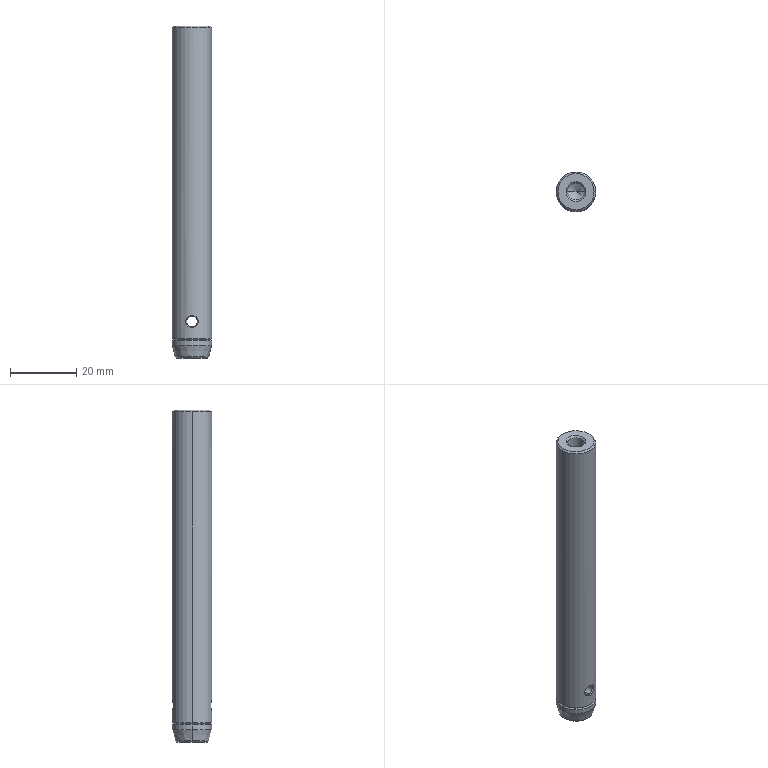Part | STEP file | 1 solid | 36 faces | box 11.9 x 11.9 x 100 mm | volume 10654 mm3 | cone 18 | cylinder 10 | spline 6 | plane 2 | commonest cylinder face diameters 11.9 x4 3.2 x2 3.3 x2 5 x2